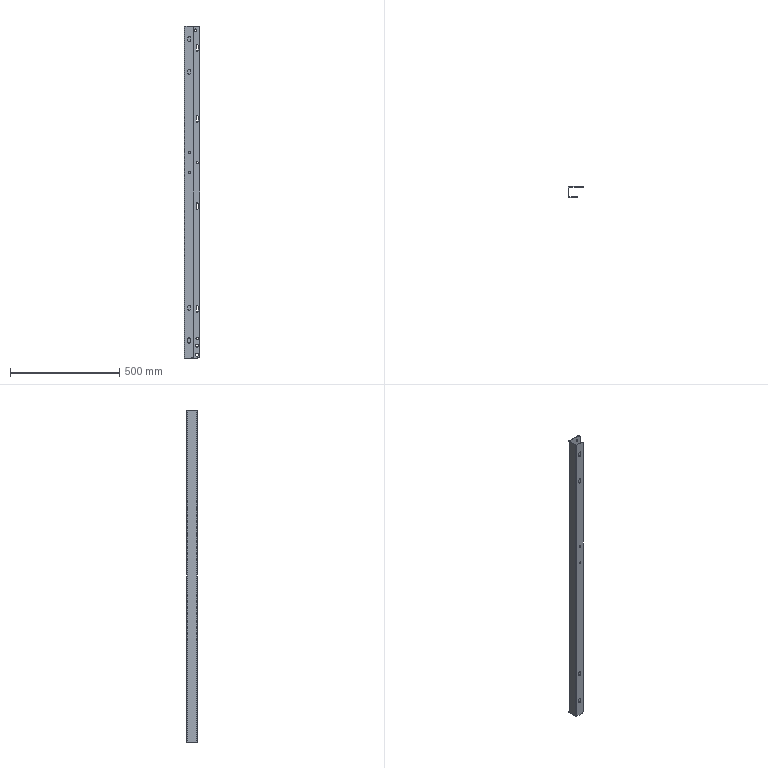Part | SolidWorks | features ICE 4, Cut 1, Fillet 1, FlatPattern 1, SMBaseFlange 1, SheetMetal 1 | 1 solid | 80 faces | box 72 x 50 x 1520 mm | volume 718399 mm3 | cylinder 42 | plane 38 | commonest cylinder face diameters 10 x14 12 x12 11 x6 24 x4 0.4 x2 6.4 x2